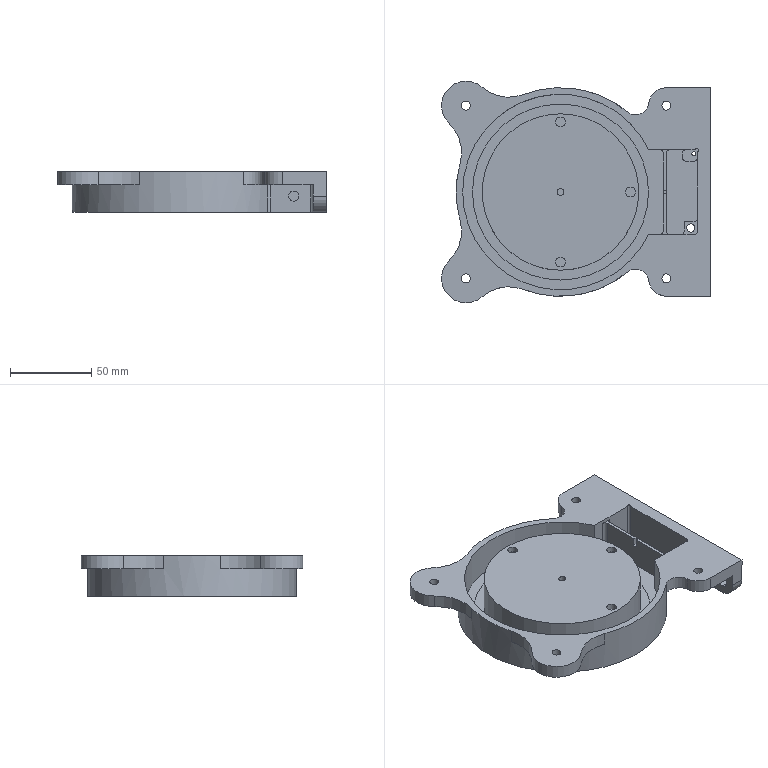Part | 2 solids | 99 faces | box 165 x 136 x 25 mm | volume 297222 mm3 | cylinder 51 | plane 48 | commonest cylinder face diameters 4 x14 6 x6 5.5 x4 7 x4 50 x4 4.2 x2